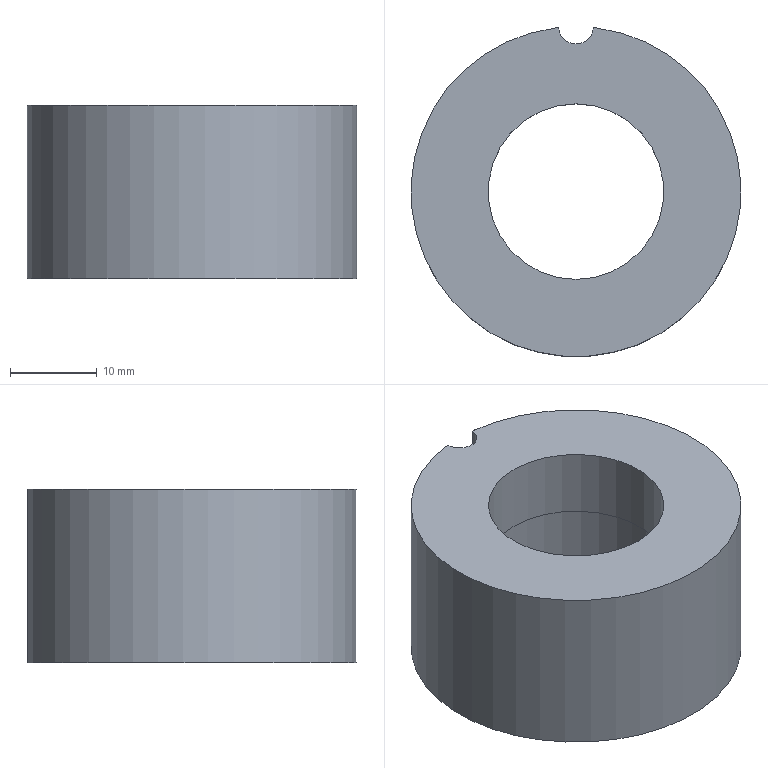Part | NX | features solid 2 | 1 solid | 9 faces | box 38 x 37.895 x 20 mm | volume 15991 mm3 | cylinder 6 | plane 3 | commonest cylinder face diameters 38 x3 4 x1 20.22 x1 20.6 x1
STEP:
#1=CARTESIAN_POINT('',(353.001,29.244,-5.264));
#2=VERTEX_POINT('',#1);
#3=CARTESIAN_POINT('',(352.628,29.201,-5.264));
#4=VERTEX_POINT('',#3);
#5=CARTESIAN_POINT('',(354.998,10.349,-5.264));
#6=DIRECTION('',(0.,0.,1.));
#7=DIRECTION('',(1.,0.,0.));
#8=AXIS2_PLACEMENT_3D('',#5,#6,#7);
#9=CIRCLE('',#8,19.);
#10=EDGE_CURVE('',#2,#4,#9,.T.);
#11=ORIENTED_EDGE('',*,*,#10,.F.);
#12=CARTESIAN_POINT('',(353.001,29.244,-25.264));
#13=VERTEX_POINT('',#12);
#14=CARTESIAN_POINT('',(353.001,29.244,-15.264));
#15=DIRECTION('',(0.,0.,1.));
#16=VECTOR('',#15,1000.);
#17=LINE('',#14,#16);
#18=EDGE_CURVE('',#2,#13,#17,.F.);
#19=ORIENTED_EDGE('',*,*,#18,.T.);
#20=CARTESIAN_POINT('',(352.628,29.201,-25.264));
#21=VERTEX_POINT('',#20);
#22=CARTESIAN_POINT('',(354.998,10.349,-25.264));
#23=DIRECTION('',(0.,0.,-1.));
#24=DIRECTION('',(-1.,0.,0.));
#25=AXIS2_PLACEMENT_3D('',#22,#23,#24);
#26=CIRCLE('',#25,19.);
#27=EDGE_CURVE('',#21,#13,#26,.T.);
#28=ORIENTED_EDGE('',*,*,#27,.F.);
#29=CARTESIAN_POINT('',(352.628,29.201,-25.264));
#30=DIRECTION('',(0.,0.,1.));
#31=VECTOR('',#30,1000.);
#32=LINE('',#29,#31);
#33=EDGE_CURVE('',#21,#4,#32,.T.);
#34=ORIENTED_EDGE('',*,*,#33,.T.);
#35=EDGE_LOOP('',(#11,#19,#28,#34));
#36=FACE_BOUND('',#35,.T.);
#37=CARTESIAN_POINT('',(354.998,10.349,-25.264));
#38=DIRECTION('',(0.,0.,1.));
#39=DIRECTION('',(0.,1.,0.));
#40=AXIS2_PLACEMENT_3D('',#37,#38,#39);
#41=CYLINDRICAL_SURFACE('',#40,19.);
#42=ADVANCED_FACE('',(#36),#41,.T.);
#43=CARTESIAN_POINT('',(356.995,29.244,-5.264));
#44=VERTEX_POINT('',#43);
#45=CARTESIAN_POINT('',(354.998,29.349,-5.264));
#46=DIRECTION('',(0.,0.,-1.));
#47=DIRECTION('',(0.,-1.,0.));
#48=AXIS2_PLACEMENT_3D('',#45,#46,#47);
#49=CIRCLE('',#48,2.);
#50=EDGE_CURVE('',#44,#2,#49,.T.);
#51=ORIENTED_EDGE('',*,*,#50,.T.);
#52=ORIENTED_EDGE('',*,*,#10,.T.);
#53=CARTESIAN_POINT('',(357.368,29.201,-5.264));
#54=VERTEX_POINT('',#53);
#55=CARTESIAN_POINT('',(354.998,10.349,-5.264));
#56=DIRECTION('',(0.,0.,1.));
#57=DIRECTION('',(1.,0.,0.));
#58=AXIS2_PLACEMENT_3D('',#55,#56,#57);
#59=CIRCLE('',#58,19.);
#60=EDGE_CURVE('',#54,#4,#59,.F.);
#61=ORIENTED_EDGE('',*,*,#60,.F.);
#62=CARTESIAN_POINT('',(354.998,10.349,-5.264));
#63=DIRECTION('',(0.,0.,1.));
#64=DIRECTION('',(1.,0.,0.));
#65=AXIS2_PLACEMENT_3D('',#62,#63,#64);
#66=CIRCLE('',#65,19.);
#67=EDGE_CURVE('',#54,#44,#66,.T.);
#68=ORIENTED_EDGE('',*,*,#67,.T.);
#69=EDGE_LOOP('',(#51,#52,#61,#68));
#70=FACE_BOUND('',#69,.T.);
#71=CARTESIAN_POINT('',(354.998,0.2393,-5.264));
#72=VERTEX_POINT('',#71);
#73=CARTESIAN_POINT('',(354.998,10.349,-5.264));
#74=DIRECTION('',(0.,0.,-1.));
#75=DIRECTION('',(0.,-1.,0.));
#76=AXIS2_PLACEMENT_3D('',#73,#74,#75);
#77=CIRCLE('',#76,10.11);
#78=EDGE_CURVE('',#72,#72,#77,.T.);
#79=ORIENTED_EDGE('',*,*,#78,.T.);
#80=EDGE_LOOP('',(#79));
#81=FACE_BOUND('',#80,.T.);
#82=CARTESIAN_POINT('',(354.998,10.349,-5.264));
#83=DIRECTION('',(0.,0.,1.));
#84=DIRECTION('',(0.,1.,0.));
#85=AXIS2_PLACEMENT_3D('',#82,#83,#84);
#86=PLANE('',#85);
#87=ADVANCED_FACE('',(#70,#81),#86,.T.);
#88=CARTESIAN_POINT('',(356.995,29.244,-25.264));
#89=VERTEX_POINT('',#88);
#90=CARTESIAN_POINT('',(354.998,29.349,-25.264));
#91=DIRECTION('',(0.,0.,1.));
#92=DIRECTION('',(0.,1.,0.));
#93=AXIS2_PLACEMENT_3D('',#90,#91,#92);
#94=CIRCLE('',#93,2.);
#95=EDGE_CURVE('',#13,#89,#94,.T.);
#96=ORIENTED_EDGE('',*,*,#95,.T.);
#97=CARTESIAN_POINT('',(357.368,29.201,-25.264));
#98=VERTEX_POINT('',#97);
#99=CARTESIAN_POINT('',(354.998,10.349,-25.264));
#100=DIRECTION('',(0.,0.,-1.));
#101=DIRECTION('',(-1.,0.,0.));
#102=AXIS2_PLACEMENT_3D('',#99,#100,#101);
#103=CIRCLE('',#102,19.);
#104=EDGE_CURVE('',#89,#98,#103,.T.);
#105=ORIENTED_EDGE('',*,*,#104,.T.);
#106=CARTESIAN_POINT('',(354.998,10.349,-25.264));
#107=DIRECTION('',(0.,0.,-1.));
#108=DIRECTION('',(-1.,0.,0.));
#109=AXIS2_PLACEMENT_3D('',#106,#107,#108);
#110=CIRCLE('',#109,19.);
#111=EDGE_CURVE('',#21,#98,#110,.F.);
#112=ORIENTED_EDGE('',*,*,#111,.F.);
#113=ORIENTED_EDGE('',*,*,#27,.T.);
#114=EDGE_LOOP('',(#96,#105,#112,#113));
#115=FACE_BOUND('',#114,.T.);
#116=CARTESIAN_POINT('',(354.998,0.04933,-25.264));
#117=VERTEX_POINT('',#116);
#118=CARTESIAN_POINT('',(354.998,10.349,-25.264));
#119=DIRECTION('',(0.,0.,-1.));
#120=DIRECTION('',(0.,-1.,0.));
#121=AXIS2_PLACEMENT_3D('',#118,#119,#120);
#122=CIRCLE('',#121,10.3);
#123=EDGE_CURVE('',#117,#117,#122,.F.);
#124=ORIENTED_EDGE('',*,*,#123,.T.);
#125=EDGE_LOOP('',(#124));
#126=FACE_BOUND('',#125,.T.);
#127=CARTESIAN_POINT('',(354.998,10.349,-25.264));
#128=DIRECTION('',(0.,0.,-1.));
#129=DIRECTION('',(0.,-1.,0.));
#130=AXIS2_PLACEMENT_3D('',#127,#128,#129);
#131=PLANE('',#130);
#132=ADVANCED_FACE('',(#115,#126),#131,.T.);
#133=ORIENTED_EDGE('',*,*,#33,.F.);
#134=ORIENTED_EDGE('',*,*,#111,.T.);
#135=CARTESIAN_POINT('',(357.368,29.201,-25.264));
#136=DIRECTION('',(0.,0.,1.));
#137=VECTOR('',#136,1000.);
#138=LINE('',#135,#137);
#139=EDGE_CURVE('',#54,#98,#138,.F.);
#140=ORIENTED_EDGE('',*,*,#139,.F.);
#141=ORIENTED_EDGE('',*,*,#60,.T.);
#142=EDGE_LOOP('',(#133,#134,#140,#141));
#143=FACE_BOUND('',#142,.T.);
#144=CARTESIAN_POINT('',(354.998,10.349,-25.264));
#145=DIRECTION('',(0.,0.,1.));
#146=DIRECTION('',(0.,1.,0.));
#147=AXIS2_PLACEMENT_3D('',#144,#145,#146);
#148=CYLINDRICAL_SURFACE('',#147,19.);
#149=ADVANCED_FACE('',(#143),#148,.T.);
#150=CARTESIAN_POINT('',(354.998,20.459,-13.264));
#151=VERTEX_POINT('',#150);
#152=CARTESIAN_POINT('',(354.998,10.349,-13.264));
#153=DIRECTION('',(0.,0.,1.));
#154=DIRECTION('',(0.,1.,0.));
#155=AXIS2_PLACEMENT_3D('',#152,#153,#154);
#156=CIRCLE('',#155,10.11);
#157=EDGE_CURVE('',#151,#151,#156,.T.);
#158=ORIENTED_EDGE('',*,*,#157,.T.);
#159=EDGE_LOOP('',(#158));
#160=FACE_BOUND('',#159,.T.);
#161=CARTESIAN_POINT('',(354.998,20.649,-13.264));
#162=VERTEX_POINT('',#161);
#163=CARTESIAN_POINT('',(354.998,10.349,-13.264));
#164=DIRECTION('',(0.,0.,1.));
#165=DIRECTION('',(0.,1.,0.));
#166=AXIS2_PLACEMENT_3D('',#163,#164,#165);
#167=CIRCLE('',#166,10.3);
#168=EDGE_CURVE('',#162,#162,#167,.F.);
#169=ORIENTED_EDGE('',*,*,#168,.T.);
#170=EDGE_LOOP('',(#169));
#171=FACE_BOUND('',#170,.T.);
#172=CARTESIAN_POINT('',(354.998,10.349,-13.264));
#173=DIRECTION('',(0.,0.,1.));
#174=DIRECTION('',(0.,1.,0.));
#175=AXIS2_PLACEMENT_3D('',#172,#173,#174);
#176=PLANE('',#175);
#177=ADVANCED_FACE('',(#160,#171),#176,.F.);
#178=ORIENTED_EDGE('',*,*,#168,.F.);
#179=EDGE_LOOP('',(#178));
#180=FACE_BOUND('',#179,.T.);
#181=ORIENTED_EDGE('',*,*,#123,.F.);
#182=EDGE_LOOP('',(#181));
#183=FACE_BOUND('',#182,.T.);
#184=CARTESIAN_POINT('',(354.998,10.349,-25.264));
#185=DIRECTION('',(0.,0.,1.));
#186=DIRECTION('',(0.,1.,0.));
#187=AXIS2_PLACEMENT_3D('',#184,#185,#186);
#188=CYLINDRICAL_SURFACE('',#187,10.3);
#189=ADVANCED_FACE('',(#180,#183),#188,.F.);
#190=ORIENTED_EDGE('',*,*,#78,.F.);
#191=EDGE_LOOP('',(#190));
#192=FACE_BOUND('',#191,.T.);
#193=ORIENTED_EDGE('',*,*,#157,.F.);
#194=EDGE_LOOP('',(#193));
#195=FACE_BOUND('',#194,.T.);
#196=CARTESIAN_POINT('',(354.998,10.349,-13.264));
#197=DIRECTION('',(0.,0.,1.));
#198=DIRECTION('',(0.,1.,0.));
#199=AXIS2_PLACEMENT_3D('',#196,#197,#198);
#200=CYLINDRICAL_SURFACE('',#199,10.11);
#201=ADVANCED_FACE('',(#192,#195),#200,.F.);
#202=ORIENTED_EDGE('',*,*,#104,.F.);
#203=CARTESIAN_POINT('',(356.995,29.244,-15.264));
#204=DIRECTION('',(0.,0.,1.));
#205=VECTOR('',#204,1000.);
#206=LINE('',#203,#205);
#207=EDGE_CURVE('',#89,#44,#206,.T.);
#208=ORIENTED_EDGE('',*,*,#207,.T.);
#209=ORIENTED_EDGE('',*,*,#67,.F.);
#210=ORIENTED_EDGE('',*,*,#139,.T.);
#211=EDGE_LOOP('',(#202,#208,#209,#210));
#212=FACE_BOUND('',#211,.T.);
#213=CARTESIAN_POINT('',(354.998,10.349,-25.264));
#214=DIRECTION('',(0.,0.,1.));
#215=DIRECTION('',(0.,1.,0.));
#216=AXIS2_PLACEMENT_3D('',#213,#214,#215);
#217=CYLINDRICAL_SURFACE('',#216,19.);
#218=ADVANCED_FACE('',(#212),#217,.T.);
#219=ORIENTED_EDGE('',*,*,#50,.F.);
#220=ORIENTED_EDGE('',*,*,#207,.F.);
#221=ORIENTED_EDGE('',*,*,#95,.F.);
#222=ORIENTED_EDGE('',*,*,#18,.F.);
#223=EDGE_LOOP('',(#219,#220,#221,#222));
#224=FACE_BOUND('',#223,.T.);
#225=CARTESIAN_POINT('',(354.998,29.349,-25.264));
#226=DIRECTION('',(0.,0.,1.));
#227=DIRECTION('',(0.,1.,0.));
#228=AXIS2_PLACEMENT_3D('',#225,#226,#227);
#229=CYLINDRICAL_SURFACE('',#228,2.);
#230=ADVANCED_FACE('',(#224),#229,.F.);
#231=CLOSED_SHELL('',(#42,#87,#132,#149,#177,#189,#201,#218,#230));
#232=MANIFOLD_SOLID_BREP('',#231);
#233=(LENGTH_UNIT()NAMED_UNIT(*)SI_UNIT(.MILLI.,.METRE.));
#234=UNCERTAINTY_MEASURE_WITH_UNIT(LENGTH_MEASURE(0.00001),#233,'','');
#235=(NAMED_UNIT(*)PLANE_ANGLE_UNIT()SI_UNIT($,.RADIAN.));
#236=(NAMED_UNIT(*)SI_UNIT($,.STERADIAN.)SOLID_ANGLE_UNIT());
#237=(GEOMETRIC_REPRESENTATION_CONTEXT(3)GLOBAL_UNCERTAINTY_ASSIGNED_CONTEXT((#234))GLOBAL_UNIT_ASSIGNED_CONTEXT((#233,#235,#236))REPRESENTATION_CONTEXT('',''));
#238=ADVANCED_BREP_SHAPE_REPRESENTATION('',(#232),#237);